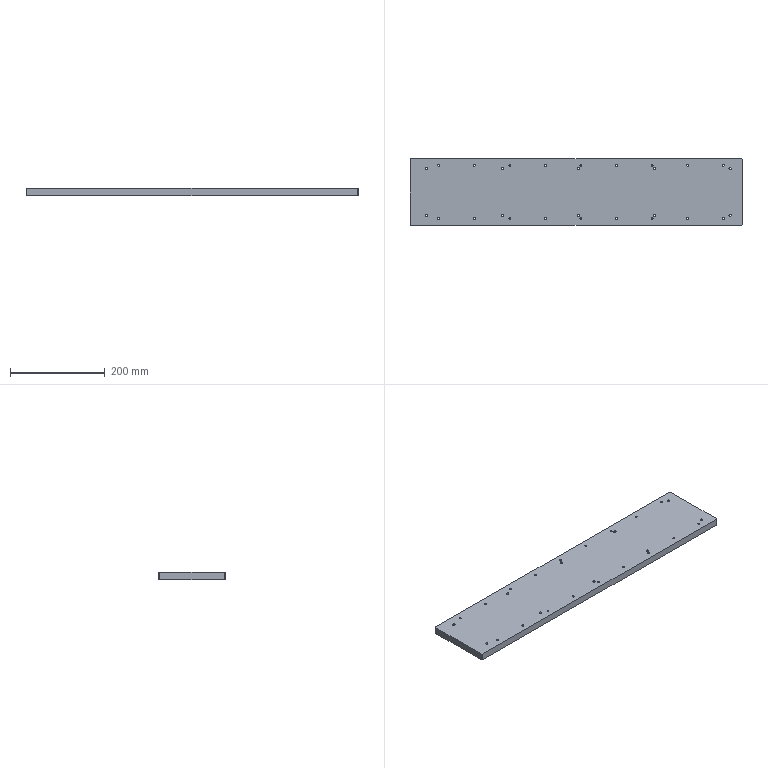Part | STEP file | 1 solid | 42 faces | box 700 x 140 x 15 mm | volume 1462585 mm3 | cylinder 30 | plane 10 | cone 2 | commonest cylinder face diameters 4.2 x18 5 x12